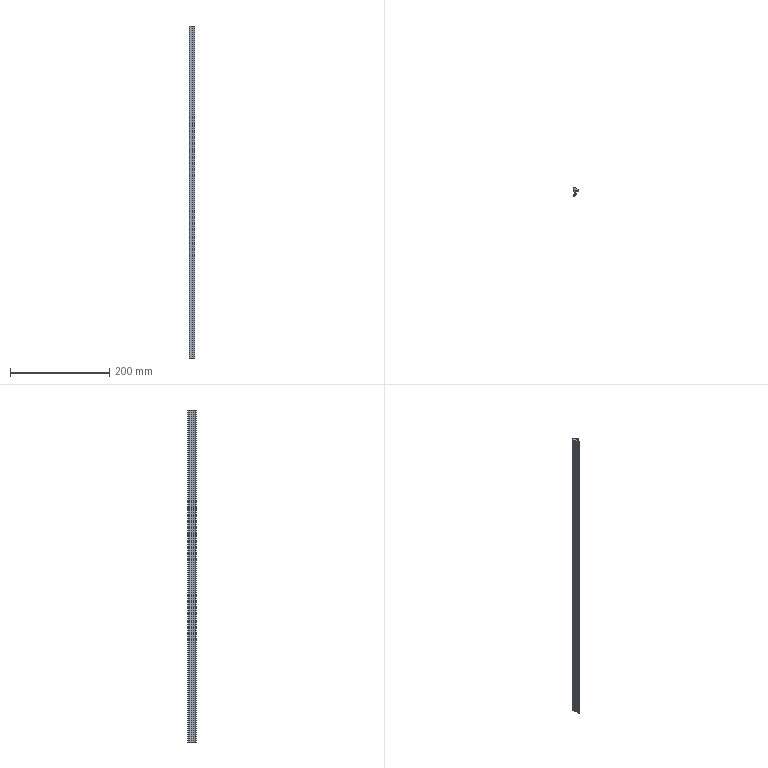Part | SolidWorks | features BaseBody 1, MoveFace 1 | 1 solid | 20 faces | box 10.8 x 17.5 x 670 mm | volume 52796 mm3 | cylinder 11 | plane 9 | commonest cylinder face diameters 1.6 x2 14 x2 0.4 x1 0.6 x1 0.8 x1 2.6 x1
STEP:
#1=CARTESIAN_POINT('',(-3.236,-11.055,570.));
#2=VERTEX_POINT('',#1);
#3=CARTESIAN_POINT('',(-4.3,-10.3,570.));
#4=VERTEX_POINT('',#3);
#5=CARTESIAN_POINT('',(-3.5,-10.3,570.));
#6=DIRECTION('',(0.,0.,-1.));
#7=DIRECTION('',(1.,0.,0.));
#8=AXIS2_PLACEMENT_3D('',#5,#6,#7);
#9=CIRCLE('',#8,0.8);
#10=EDGE_CURVE('',#2,#4,#9,.T.);
#11=ORIENTED_EDGE('',*,*,#10,.T.);
#12=CARTESIAN_POINT('',(-4.3,-10.3,-100.));
#13=VERTEX_POINT('',#12);
#14=CARTESIAN_POINT('',(-4.3,-10.3,-100.));
#15=DIRECTION('',(0.,0.,-1.));
#16=VECTOR('',#15,1000.);
#17=LINE('',#14,#16);
#18=EDGE_CURVE('',#4,#13,#17,.T.);
#19=ORIENTED_EDGE('',*,*,#18,.T.);
#20=CARTESIAN_POINT('',(-3.236,-11.055,-100.));
#21=VERTEX_POINT('',#20);
#22=CARTESIAN_POINT('',(-3.5,-10.3,-100.));
#23=DIRECTION('',(0.,0.,1.));
#24=DIRECTION('',(-1.,0.,0.));
#25=AXIS2_PLACEMENT_3D('',#22,#23,#24);
#26=CIRCLE('',#25,0.8);
#27=EDGE_CURVE('',#13,#21,#26,.T.);
#28=ORIENTED_EDGE('',*,*,#27,.T.);
#29=CARTESIAN_POINT('',(-3.236,-11.055,-100.));
#30=DIRECTION('',(0.,0.,-1.));
#31=VECTOR('',#30,1000.);
#32=LINE('',#29,#31);
#33=EDGE_CURVE('',#2,#21,#32,.T.);
#34=ORIENTED_EDGE('',*,*,#33,.F.);
#35=EDGE_LOOP('',(#11,#19,#28,#34));
#36=FACE_OUTER_BOUND('',#35,.T.);
#37=CARTESIAN_POINT('',(-3.5,-10.3,-100.));
#38=DIRECTION('',(0.,0.,-1.));
#39=DIRECTION('',(-1.,0.,0.));
#40=AXIS2_PLACEMENT_3D('',#37,#38,#39);
#41=CYLINDRICAL_SURFACE('',#40,0.8);
#42=ADVANCED_FACE('',(#36),#41,.T.);
#43=CARTESIAN_POINT('',(1.184,-6.397,-100.));
#44=VERTEX_POINT('',#43);
#45=CARTESIAN_POINT('',(-5.702,-4.29,-100.));
#46=DIRECTION('',(0.,0.,1.));
#47=DIRECTION('',(-1.,0.,0.));
#48=AXIS2_PLACEMENT_3D('',#45,#46,#47);
#49=CIRCLE('',#48,7.201);
#50=EDGE_CURVE('',#21,#44,#49,.T.);
#51=ORIENTED_EDGE('',*,*,#50,.T.);
#52=CARTESIAN_POINT('',(1.184,-6.397,570.));
#53=VERTEX_POINT('',#52);
#54=CARTESIAN_POINT('',(1.184,-6.397,-100.));
#55=DIRECTION('',(0.,0.,1.));
#56=VECTOR('',#55,1000.);
#57=LINE('',#54,#56);
#58=EDGE_CURVE('',#44,#53,#57,.T.);
#59=ORIENTED_EDGE('',*,*,#58,.T.);
#60=CARTESIAN_POINT('',(-5.702,-4.29,570.));
#61=DIRECTION('',(0.,0.,-1.));
#62=DIRECTION('',(1.,0.,0.));
#63=AXIS2_PLACEMENT_3D('',#60,#61,#62);
#64=CIRCLE('',#63,7.201);
#65=EDGE_CURVE('',#53,#2,#64,.T.);
#66=ORIENTED_EDGE('',*,*,#65,.T.);
#67=ORIENTED_EDGE('',*,*,#33,.T.);
#68=EDGE_LOOP('',(#51,#59,#66,#67));
#69=FACE_OUTER_BOUND('',#68,.T.);
#70=CARTESIAN_POINT('',(-5.702,-4.29,-100.));
#71=DIRECTION('',(0.,0.,-1.));
#72=DIRECTION('',(-1.,0.,0.));
#73=AXIS2_PLACEMENT_3D('',#70,#71,#72);
#74=CYLINDRICAL_SURFACE('',#73,7.201);
#75=ADVANCED_FACE('',(#69),#74,.T.);
#76=CARTESIAN_POINT('',(0.9,-6.,-100.));
#77=VERTEX_POINT('',#76);
#78=CARTESIAN_POINT('',(0.9,-6.3,-100.));
#79=DIRECTION('',(0.,0.,1.));
#80=DIRECTION('',(-1.,0.,0.));
#81=AXIS2_PLACEMENT_3D('',#78,#79,#80);
#82=CIRCLE('',#81,0.3);
#83=EDGE_CURVE('',#44,#77,#82,.T.);
#84=ORIENTED_EDGE('',*,*,#83,.T.);
#85=CARTESIAN_POINT('',(0.9,-6.,570.));
#86=VERTEX_POINT('',#85);
#87=CARTESIAN_POINT('',(0.9,-6.,-100.));
#88=DIRECTION('',(0.,0.,1.));
#89=VECTOR('',#88,1000.);
#90=LINE('',#87,#89);
#91=EDGE_CURVE('',#77,#86,#90,.T.);
#92=ORIENTED_EDGE('',*,*,#91,.T.);
#93=CARTESIAN_POINT('',(0.9,-6.3,570.));
#94=DIRECTION('',(0.,0.,-1.));
#95=DIRECTION('',(1.,0.,0.));
#96=AXIS2_PLACEMENT_3D('',#93,#94,#95);
#97=CIRCLE('',#96,0.3);
#98=EDGE_CURVE('',#86,#53,#97,.T.);
#99=ORIENTED_EDGE('',*,*,#98,.T.);
#100=ORIENTED_EDGE('',*,*,#58,.F.);
#101=EDGE_LOOP('',(#84,#92,#99,#100));
#102=FACE_OUTER_BOUND('',#101,.T.);
#103=CARTESIAN_POINT('',(0.9,-6.3,-100.));
#104=DIRECTION('',(0.,0.,-1.));
#105=DIRECTION('',(-1.,0.,0.));
#106=AXIS2_PLACEMENT_3D('',#103,#104,#105);
#107=CYLINDRICAL_SURFACE('',#106,0.3);
#108=ADVANCED_FACE('',(#102),#107,.T.);
#109=CARTESIAN_POINT('',(-2.5,-0.5,-100.));
#110=VERTEX_POINT('',#109);
#111=CARTESIAN_POINT('',(-2.5,-6.153,-100.));
#112=VERTEX_POINT('',#111);
#113=CARTESIAN_POINT('',(-2.5,-6.397,-100.));
#114=DIRECTION('',(0.,-1.,0.));
#115=VECTOR('',#114,1000.);
#116=LINE('',#113,#115);
#117=EDGE_CURVE('',#110,#112,#116,.T.);
#118=ORIENTED_EDGE('',*,*,#117,.F.);
#119=CARTESIAN_POINT('',(-4.2,1.695,-100.));
#120=VERTEX_POINT('',#119);
#121=CARTESIAN_POINT('',(-1.701,1.875,-100.));
#122=DIRECTION('',(0.,0.,1.));
#123=DIRECTION('',(-1.,0.,0.));
#124=AXIS2_PLACEMENT_3D('',#121,#122,#123);
#125=CIRCLE('',#124,2.506);
#126=EDGE_CURVE('',#120,#110,#125,.T.);
#127=ORIENTED_EDGE('',*,*,#126,.F.);
#128=CARTESIAN_POINT('',(-4.2,5.1,-100.));
#129=VERTEX_POINT('',#128);
#130=CARTESIAN_POINT('',(-4.2,-6.397,-100.));
#131=DIRECTION('',(0.,-1.,0.));
#132=VECTOR('',#131,1000.);
#133=LINE('',#130,#132);
#134=EDGE_CURVE('',#129,#120,#133,.T.);
#135=ORIENTED_EDGE('',*,*,#134,.F.);
#136=CARTESIAN_POINT('',(-2.892,6.4,-100.));
#137=VERTEX_POINT('',#136);
#138=CARTESIAN_POINT('',(-2.9,5.1,-100.));
#139=DIRECTION('',(0.,0.,1.));
#140=DIRECTION('',(-1.,0.,0.));
#141=AXIS2_PLACEMENT_3D('',#138,#139,#140);
#142=CIRCLE('',#141,1.3);
#143=EDGE_CURVE('',#137,#129,#142,.T.);
#144=ORIENTED_EDGE('',*,*,#143,.F.);
#145=CARTESIAN_POINT('',(0.5,5.5,-100.));
#146=VERTEX_POINT('',#145);
#147=CARTESIAN_POINT('',(-2.934,-0.5999,-100.));
#148=DIRECTION('',(0.,0.,1.));
#149=DIRECTION('',(-1.,0.,0.));
#150=AXIS2_PLACEMENT_3D('',#147,#148,#149);
#151=CIRCLE('',#150,7.);
#152=EDGE_CURVE('',#146,#137,#151,.T.);
#153=ORIENTED_EDGE('',*,*,#152,.F.);
#154=CARTESIAN_POINT('',(5.5,1.7,-100.));
#155=VERTEX_POINT('',#154);
#156=CARTESIAN_POINT('',(5.5,1.7,-100.));
#157=DIRECTION('',(-0.7962,0.6051,0.));
#158=VECTOR('',#157,1000.);
#159=LINE('',#156,#158);
#160=EDGE_CURVE('',#155,#146,#159,.T.);
#161=ORIENTED_EDGE('',*,*,#160,.F.);
#162=CARTESIAN_POINT('',(6.458,-0.2215,-100.));
#163=VERTEX_POINT('',#162);
#164=CARTESIAN_POINT('',(6.458,-0.2215,-100.));
#165=DIRECTION('',(-0.4462,0.8949,0.));
#166=VECTOR('',#165,1000.);
#167=LINE('',#164,#166);
#168=EDGE_CURVE('',#163,#155,#167,.T.);
#169=ORIENTED_EDGE('',*,*,#168,.F.);
#170=CARTESIAN_POINT('',(5.895,-0.7433,-100.));
#171=VERTEX_POINT('',#170);
#172=CARTESIAN_POINT('',(6.1,-0.4,-100.));
#173=DIRECTION('',(0.,0.,1.));
#174=DIRECTION('',(-1.,0.,0.));
#175=AXIS2_PLACEMENT_3D('',#172,#173,#174);
#176=CIRCLE('',#175,0.4);
#177=EDGE_CURVE('',#171,#163,#176,.T.);
#178=ORIENTED_EDGE('',*,*,#177,.F.);
#179=CARTESIAN_POINT('',(3.,0.,-100.));
#180=VERTEX_POINT('',#179);
#181=CARTESIAN_POINT('',(2.746,-6.995,-100.));
#182=DIRECTION('',(0.,0.,-1.));
#183=DIRECTION('',(-1.,0.,0.));
#184=AXIS2_PLACEMENT_3D('',#181,#182,#183);
#185=CIRCLE('',#184,7.);
#186=EDGE_CURVE('',#180,#171,#185,.T.);
#187=ORIENTED_EDGE('',*,*,#186,.F.);
#188=CARTESIAN_POINT('',(0.,0.,-100.));
#189=VERTEX_POINT('',#188);
#190=CARTESIAN_POINT('',(-6.814,0.,-100.));
#191=DIRECTION('',(1.,0.,0.));
#192=VECTOR('',#191,1000.);
#193=LINE('',#190,#192);
#194=EDGE_CURVE('',#189,#180,#193,.T.);
#195=ORIENTED_EDGE('',*,*,#194,.F.);
#196=CARTESIAN_POINT('',(0.,-5.8,-100.));
#197=VERTEX_POINT('',#196);
#198=CARTESIAN_POINT('',(0.,-6.397,-100.));
#199=DIRECTION('',(0.,1.,0.));
#200=VECTOR('',#199,1000.);
#201=LINE('',#198,#200);
#202=EDGE_CURVE('',#197,#189,#201,.T.);
#203=ORIENTED_EDGE('',*,*,#202,.F.);
#204=CARTESIAN_POINT('',(0.2,-6.,-100.));
#205=VERTEX_POINT('',#204);
#206=CARTESIAN_POINT('',(0.2,-5.8,-100.));
#207=DIRECTION('',(0.,0.,1.));
#208=DIRECTION('',(-1.,0.,0.));
#209=AXIS2_PLACEMENT_3D('',#206,#207,#208);
#210=CIRCLE('',#209,0.2);
#211=EDGE_CURVE('',#197,#205,#210,.T.);
#212=ORIENTED_EDGE('',*,*,#211,.T.);
#213=CARTESIAN_POINT('',(-6.814,-6.,-100.));
#214=DIRECTION('',(-1.,0.,0.));
#215=VECTOR('',#214,1000.);
#216=LINE('',#213,#215);
#217=EDGE_CURVE('',#77,#205,#216,.T.);
#218=ORIENTED_EDGE('',*,*,#217,.F.);
#219=ORIENTED_EDGE('',*,*,#83,.F.);
#220=ORIENTED_EDGE('',*,*,#50,.F.);
#221=ORIENTED_EDGE('',*,*,#27,.F.);
#222=CARTESIAN_POINT('',(-3.998,-9.674,-100.));
#223=VERTEX_POINT('',#222);
#224=CARTESIAN_POINT('',(-3.5,-10.3,-100.));
#225=DIRECTION('',(0.,0.,1.));
#226=DIRECTION('',(-1.,0.,0.));
#227=AXIS2_PLACEMENT_3D('',#224,#225,#226);
#228=CIRCLE('',#227,0.8);
#229=EDGE_CURVE('',#223,#13,#228,.T.);
#230=ORIENTED_EDGE('',*,*,#229,.F.);
#231=CARTESIAN_POINT('',(-6.814,-6.397,-100.));
#232=DIRECTION('',(0.,0.,-1.));
#233=DIRECTION('',(-1.,0.,0.));
#234=AXIS2_PLACEMENT_3D('',#231,#232,#233);
#235=CIRCLE('',#234,4.321);
#236=EDGE_CURVE('',#112,#223,#235,.T.);
#237=ORIENTED_EDGE('',*,*,#236,.F.);
#238=EDGE_LOOP('',(#118,#127,#135,#144,#153,#161,#169,#178,#187,#195,#203,#212,#218,#219,#220,#221,#230,#237));
#239=FACE_OUTER_BOUND('',#238,.T.);
#240=CARTESIAN_POINT('',(-6.814,-6.397,-100.));
#241=DIRECTION('',(0.,0.,1.));
#242=DIRECTION('',(1.,0.,0.));
#243=AXIS2_PLACEMENT_3D('',#240,#241,#242);
#244=PLANE('',#243);
#245=ADVANCED_FACE('',(#239),#244,.F.);
#246=ORIENTED_EDGE('',*,*,#18,.F.);
#247=CARTESIAN_POINT('',(-3.998,-9.674,570.));
#248=VERTEX_POINT('',#247);
#249=CARTESIAN_POINT('',(-3.5,-10.3,570.));
#250=DIRECTION('',(0.,0.,-1.));
#251=DIRECTION('',(1.,0.,0.));
#252=AXIS2_PLACEMENT_3D('',#249,#250,#251);
#253=CIRCLE('',#252,0.8);
#254=EDGE_CURVE('',#4,#248,#253,.T.);
#255=ORIENTED_EDGE('',*,*,#254,.T.);
#256=CARTESIAN_POINT('',(-3.998,-9.674,-100.));
#257=DIRECTION('',(0.,0.,-1.));
#258=VECTOR('',#257,1000.);
#259=LINE('',#256,#258);
#260=EDGE_CURVE('',#248,#223,#259,.T.);
#261=ORIENTED_EDGE('',*,*,#260,.T.);
#262=ORIENTED_EDGE('',*,*,#229,.T.);
#263=EDGE_LOOP('',(#246,#255,#261,#262));
#264=FACE_OUTER_BOUND('',#263,.T.);
#265=CARTESIAN_POINT('',(-3.5,-10.3,-100.));
#266=DIRECTION('',(0.,0.,-1.));
#267=DIRECTION('',(-1.,0.,0.));
#268=AXIS2_PLACEMENT_3D('',#265,#266,#267);
#269=CYLINDRICAL_SURFACE('',#268,0.8);
#270=ADVANCED_FACE('',(#264),#269,.T.);
#271=CARTESIAN_POINT('',(-4.2,1.695,570.));
#272=VERTEX_POINT('',#271);
#273=CARTESIAN_POINT('',(-2.5,-0.5,570.));
#274=VERTEX_POINT('',#273);
#275=CARTESIAN_POINT('',(-1.701,1.875,570.));
#276=DIRECTION('',(0.,0.,1.));
#277=DIRECTION('',(1.,0.,0.));
#278=AXIS2_PLACEMENT_3D('',#275,#276,#277);
#279=CIRCLE('',#278,2.506);
#280=EDGE_CURVE('',#272,#274,#279,.T.);
#281=ORIENTED_EDGE('',*,*,#280,.T.);
#282=CARTESIAN_POINT('',(-2.5,-6.153,570.));
#283=VERTEX_POINT('',#282);
#284=CARTESIAN_POINT('',(-2.5,-6.397,570.));
#285=DIRECTION('',(0.,-1.,0.));
#286=VECTOR('',#285,1000.);
#287=LINE('',#284,#286);
#288=EDGE_CURVE('',#274,#283,#287,.T.);
#289=ORIENTED_EDGE('',*,*,#288,.T.);
#290=CARTESIAN_POINT('',(-6.814,-6.397,570.));
#291=DIRECTION('',(0.,0.,-1.));
#292=DIRECTION('',(1.,0.,0.));
#293=AXIS2_PLACEMENT_3D('',#290,#291,#292);
#294=CIRCLE('',#293,4.321);
#295=EDGE_CURVE('',#283,#248,#294,.T.);
#296=ORIENTED_EDGE('',*,*,#295,.T.);
#297=ORIENTED_EDGE('',*,*,#254,.F.);
#298=ORIENTED_EDGE('',*,*,#10,.F.);
#299=ORIENTED_EDGE('',*,*,#65,.F.);
#300=ORIENTED_EDGE('',*,*,#98,.F.);
#301=CARTESIAN_POINT('',(0.2,-6.,570.));
#302=VERTEX_POINT('',#301);
#303=CARTESIAN_POINT('',(-6.814,-6.,570.));
#304=DIRECTION('',(-1.,0.,0.));
#305=VECTOR('',#304,1000.);
#306=LINE('',#303,#305);
#307=EDGE_CURVE('',#86,#302,#306,.T.);
#308=ORIENTED_EDGE('',*,*,#307,.T.);
#309=CARTESIAN_POINT('',(0.,-5.8,570.));
#310=VERTEX_POINT('',#309);
#311=CARTESIAN_POINT('',(0.2,-5.8,570.));
#312=DIRECTION('',(0.,0.,-1.));
#313=DIRECTION('',(1.,0.,0.));
#314=AXIS2_PLACEMENT_3D('',#311,#312,#313);
#315=CIRCLE('',#314,0.2);
#316=EDGE_CURVE('',#302,#310,#315,.T.);
#317=ORIENTED_EDGE('',*,*,#316,.T.);
#318=CARTESIAN_POINT('',(0.,0.,570.));
#319=VERTEX_POINT('',#318);
#320=CARTESIAN_POINT('',(0.,-6.397,570.));
#321=DIRECTION('',(0.,1.,0.));
#322=VECTOR('',#321,1000.);
#323=LINE('',#320,#322);
#324=EDGE_CURVE('',#310,#319,#323,.T.);
#325=ORIENTED_EDGE('',*,*,#324,.T.);
#326=CARTESIAN_POINT('',(3.,0.,570.));
#327=VERTEX_POINT('',#326);
#328=CARTESIAN_POINT('',(-6.814,0.,570.));
#329=DIRECTION('',(1.,0.,0.));
#330=VECTOR('',#329,1000.);
#331=LINE('',#328,#330);
#332=EDGE_CURVE('',#319,#327,#331,.T.);
#333=ORIENTED_EDGE('',*,*,#332,.T.);
#334=CARTESIAN_POINT('',(5.895,-0.7433,570.));
#335=VERTEX_POINT('',#334);
#336=CARTESIAN_POINT('',(2.746,-6.995,570.));
#337=DIRECTION('',(0.,0.,-1.));
#338=DIRECTION('',(1.,0.,0.));
#339=AXIS2_PLACEMENT_3D('',#336,#337,#338);
#340=CIRCLE('',#339,7.);
#341=EDGE_CURVE('',#327,#335,#340,.T.);
#342=ORIENTED_EDGE('',*,*,#341,.T.);
#343=CARTESIAN_POINT('',(6.458,-0.2215,570.));
#344=VERTEX_POINT('',#343);
#345=CARTESIAN_POINT('',(6.1,-0.4,570.));
#346=DIRECTION('',(0.,0.,-1.));
#347=DIRECTION('',(1.,0.,0.));
#348=AXIS2_PLACEMENT_3D('',#345,#346,#347);
#349=CIRCLE('',#348,0.4);
#350=EDGE_CURVE('',#344,#335,#349,.T.);
#351=ORIENTED_EDGE('',*,*,#350,.F.);
#352=CARTESIAN_POINT('',(5.5,1.7,570.));
#353=VERTEX_POINT('',#352);
#354=CARTESIAN_POINT('',(6.282,0.1323,570.));
#355=DIRECTION('',(-0.4462,0.8949,0.));
#356=VECTOR('',#355,1000.);
#357=LINE('',#354,#356);
#358=EDGE_CURVE('',#344,#353,#357,.T.);
#359=ORIENTED_EDGE('',*,*,#358,.T.);
#360=CARTESIAN_POINT('',(0.5,5.5,570.));
#361=VERTEX_POINT('',#360);
#362=CARTESIAN_POINT('',(1.595,4.668,570.));
#363=DIRECTION('',(-0.7962,0.6051,0.));
#364=VECTOR('',#363,1000.);
#365=LINE('',#362,#364);
#366=EDGE_CURVE('',#353,#361,#365,.T.);
#367=ORIENTED_EDGE('',*,*,#366,.T.);
#368=CARTESIAN_POINT('',(-2.892,6.4,570.));
#369=VERTEX_POINT('',#368);
#370=CARTESIAN_POINT('',(-2.934,-0.5999,570.));
#371=DIRECTION('',(0.,0.,1.));
#372=DIRECTION('',(1.,0.,0.));
#373=AXIS2_PLACEMENT_3D('',#370,#371,#372);
#374=CIRCLE('',#373,7.);
#375=EDGE_CURVE('',#361,#369,#374,.T.);
#376=ORIENTED_EDGE('',*,*,#375,.T.);
#377=CARTESIAN_POINT('',(-4.2,5.1,570.));
#378=VERTEX_POINT('',#377);
#379=CARTESIAN_POINT('',(-2.9,5.1,570.));
#380=DIRECTION('',(0.,0.,1.));
#381=DIRECTION('',(1.,0.,0.));
#382=AXIS2_PLACEMENT_3D('',#379,#380,#381);
#383=CIRCLE('',#382,1.3);
#384=EDGE_CURVE('',#369,#378,#383,.T.);
#385=ORIENTED_EDGE('',*,*,#384,.T.);
#386=CARTESIAN_POINT('',(-4.2,-6.397,570.));
#387=DIRECTION('',(0.,-1.,0.));
#388=VECTOR('',#387,1000.);
#389=LINE('',#386,#388);
#390=EDGE_CURVE('',#378,#272,#389,.T.);
#391=ORIENTED_EDGE('',*,*,#390,.T.);
#392=EDGE_LOOP('',(#281,#289,#296,#297,#298,#299,#300,#308,#317,#325,#333,#342,#351,#359,#367,#376,#385,#391));
#393=FACE_OUTER_BOUND('',#392,.T.);
#394=CARTESIAN_POINT('',(-6.814,-6.397,570.));
#395=DIRECTION('',(0.,0.,1.));
#396=DIRECTION('',(1.,0.,0.));
#397=AXIS2_PLACEMENT_3D('',#394,#395,#396);
#398=PLANE('',#397);
#399=ADVANCED_FACE('',(#393),#398,.T.);
#400=ORIENTED_EDGE('',*,*,#217,.T.);
#401=CARTESIAN_POINT('',(0.2,-6.,-100.));
#402=DIRECTION('',(0.,0.,1.));
#403=VECTOR('',#402,1000.);
#404=LINE('',#401,#403);
#405=EDGE_CURVE('',#205,#302,#404,.T.);
#406=ORIENTED_EDGE('',*,*,#405,.T.);
#407=ORIENTED_EDGE('',*,*,#307,.F.);
#408=ORIENTED_EDGE('',*,*,#91,.F.);
#409=EDGE_LOOP('',(#400,#406,#407,#408));
#410=FACE_OUTER_BOUND('',#409,.T.);
#411=CARTESIAN_POINT('',(0.9,-6.,-100.));
#412=DIRECTION('',(0.,1.,0.));
#413=DIRECTION('',(0.,0.,1.));
#414=AXIS2_PLACEMENT_3D('',#411,#412,#413);
#415=PLANE('',#414);
#416=ADVANCED_FACE('',(#410),#415,.T.);
#417=CARTESIAN_POINT('',(-2.5,-6.153,-100.));
#418=DIRECTION('',(0.,0.,1.));
#419=VECTOR('',#418,1000.);
#420=LINE('',#417,#419);
#421=EDGE_CURVE('',#112,#283,#420,.T.);
#422=ORIENTED_EDGE('',*,*,#421,.F.);
#423=ORIENTED_EDGE('',*,*,#236,.T.);
#424=ORIENTED_EDGE('',*,*,#260,.F.);
#425=ORIENTED_EDGE('',*,*,#295,.F.);
#426=EDGE_LOOP('',(#422,#423,#424,#425));
#427=FACE_OUTER_BOUND('',#426,.T.);
#428=CARTESIAN_POINT('',(-6.814,-6.397,-100.));
#429=DIRECTION('',(0.,0.,-1.));
#430=DIRECTION('',(-1.,0.,0.));
#431=AXIS2_PLACEMENT_3D('',#428,#429,#430);
#432=CYLINDRICAL_SURFACE('',#431,4.321);
#433=ADVANCED_FACE('',(#427),#432,.F.);
#434=ORIENTED_EDGE('',*,*,#117,.T.);
#435=ORIENTED_EDGE('',*,*,#421,.T.);
#436=ORIENTED_EDGE('',*,*,#288,.F.);
#437=CARTESIAN_POINT('',(-2.5,-0.5,-100.));
#438=DIRECTION('',(0.,0.,-1.));
#439=VECTOR('',#438,1000.);
#440=LINE('',#437,#439);
#441=EDGE_CURVE('',#274,#110,#440,.T.);
#442=ORIENTED_EDGE('',*,*,#441,.T.);
#443=EDGE_LOOP('',(#434,#435,#436,#442));
#444=FACE_OUTER_BOUND('',#443,.T.);
#445=CARTESIAN_POINT('',(-2.5,-0.5,-100.));
#446=DIRECTION('',(-1.,0.,0.));
#447=DIRECTION('',(0.,0.,1.));
#448=AXIS2_PLACEMENT_3D('',#445,#446,#447);
#449=PLANE('',#448);
#450=ADVANCED_FACE('',(#444),#449,.T.);
#451=ORIENTED_EDGE('',*,*,#126,.T.);
#452=ORIENTED_EDGE('',*,*,#441,.F.);
#453=ORIENTED_EDGE('',*,*,#280,.F.);
#454=CARTESIAN_POINT('',(-4.2,1.695,-100.));
#455=DIRECTION('',(0.,0.,-1.));
#456=VECTOR('',#455,1000.);
#457=LINE('',#454,#456);
#458=EDGE_CURVE('',#272,#120,#457,.T.);
#459=ORIENTED_EDGE('',*,*,#458,.T.);
#460=EDGE_LOOP('',(#451,#452,#453,#459));
#461=FACE_OUTER_BOUND('',#460,.T.);
#462=CARTESIAN_POINT('',(-1.701,1.875,-100.));
#463=DIRECTION('',(0.,0.,-1.));
#464=DIRECTION('',(-1.,0.,0.));
#465=AXIS2_PLACEMENT_3D('',#462,#463,#464);
#466=CYLINDRICAL_SURFACE('',#465,2.506);
#467=ADVANCED_FACE('',(#461),#466,.T.);
#468=ORIENTED_EDGE('',*,*,#134,.T.);
#469=ORIENTED_EDGE('',*,*,#458,.F.);
#470=ORIENTED_EDGE('',*,*,#390,.F.);
#471=CARTESIAN_POINT('',(-4.2,5.1,-100.));
#472=DIRECTION('',(0.,0.,-1.));
#473=VECTOR('',#472,1000.);
#474=LINE('',#471,#473);
#475=EDGE_CURVE('',#378,#129,#474,.T.);
#476=ORIENTED_EDGE('',*,*,#475,.T.);
#477=EDGE_LOOP('',(#468,#469,#470,#476));
#478=FACE_OUTER_BOUND('',#477,.T.);
#479=CARTESIAN_POINT('',(-4.2,5.1,-100.));
#480=DIRECTION('',(-1.,0.,0.));
#481=DIRECTION('',(0.,0.,1.));
#482=AXIS2_PLACEMENT_3D('',#479,#480,#481);
#483=PLANE('',#482);
#484=ADVANCED_FACE('',(#478),#483,.T.);
#485=ORIENTED_EDGE('',*,*,#143,.T.);
#486=ORIENTED_EDGE('',*,*,#475,.F.);
#487=ORIENTED_EDGE('',*,*,#384,.F.);
#488=CARTESIAN_POINT('',(-2.892,6.4,-100.));
#489=DIRECTION('',(0.,0.,-1.));
#490=VECTOR('',#489,1000.);
#491=LINE('',#488,#490);
#492=EDGE_CURVE('',#369,#137,#491,.T.);
#493=ORIENTED_EDGE('',*,*,#492,.T.);
#494=EDGE_LOOP('',(#485,#486,#487,#493));
#495=FACE_OUTER_BOUND('',#494,.T.);
#496=CARTESIAN_POINT('',(-2.9,5.1,-100.));
#497=DIRECTION('',(0.,0.,-1.));
#498=DIRECTION('',(-1.,0.,0.));
#499=AXIS2_PLACEMENT_3D('',#496,#497,#498);
#500=CYLINDRICAL_SURFACE('',#499,1.3);
#501=ADVANCED_FACE('',(#495),#500,.T.);
#502=ORIENTED_EDGE('',*,*,#152,.T.);
#503=ORIENTED_EDGE('',*,*,#492,.F.);
#504=ORIENTED_EDGE('',*,*,#375,.F.);
#505=CARTESIAN_POINT('',(0.5,5.5,-100.));
#506=DIRECTION('',(0.,0.,-1.));
#507=VECTOR('',#506,1000.);
#508=LINE('',#505,#507);
#509=EDGE_CURVE('',#361,#146,#508,.T.);
#510=ORIENTED_EDGE('',*,*,#509,.T.);
#511=EDGE_LOOP('',(#502,#503,#504,#510));
#512=FACE_OUTER_BOUND('',#511,.T.);
#513=CARTESIAN_POINT('',(-2.934,-0.5999,-100.));
#514=DIRECTION('',(0.,0.,-1.));
#515=DIRECTION('',(-1.,0.,0.));
#516=AXIS2_PLACEMENT_3D('',#513,#514,#515);
#517=CYLINDRICAL_SURFACE('',#516,7.);
#518=ADVANCED_FACE('',(#512),#517,.T.);
#519=ORIENTED_EDGE('',*,*,#160,.T.);
#520=ORIENTED_EDGE('',*,*,#509,.F.);
#521=ORIENTED_EDGE('',*,*,#366,.F.);
#522=CARTESIAN_POINT('',(5.5,1.7,-100.));
#523=DIRECTION('',(0.,0.,-1.));
#524=VECTOR('',#523,1000.);
#525=LINE('',#522,#524);
#526=EDGE_CURVE('',#353,#155,#525,.T.);
#527=ORIENTED_EDGE('',*,*,#526,.T.);
#528=EDGE_LOOP('',(#519,#520,#521,#527));
#529=FACE_OUTER_BOUND('',#528,.T.);
#530=CARTESIAN_POINT('',(5.5,1.7,-100.));
#531=DIRECTION('',(0.6051,0.7962,0.));
#532=DIRECTION('',(-0.7962,0.6051,0.));
#533=AXIS2_PLACEMENT_3D('',#530,#531,#532);
#534=PLANE('',#533);
#535=ADVANCED_FACE('',(#529),#534,.T.);
#536=ORIENTED_EDGE('',*,*,#168,.T.);
#537=ORIENTED_EDGE('',*,*,#526,.F.);
#538=ORIENTED_EDGE('',*,*,#358,.F.);
#539=CARTESIAN_POINT('',(6.458,-0.2215,-100.));
#540=DIRECTION('',(0.,0.,-1.));
#541=VECTOR('',#540,1000.);
#542=LINE('',#539,#541);
#543=EDGE_CURVE('',#344,#163,#542,.T.);
#544=ORIENTED_EDGE('',*,*,#543,.T.);
#545=EDGE_LOOP('',(#536,#537,#538,#544));
#546=FACE_OUTER_BOUND('',#545,.T.);
#547=CARTESIAN_POINT('',(6.458,-0.2215,-100.));
#548=DIRECTION('',(0.8949,0.4462,0.));
#549=DIRECTION('',(-0.4462,0.8949,0.));
#550=AXIS2_PLACEMENT_3D('',#547,#548,#549);
#551=PLANE('',#550);
#552=ADVANCED_FACE('',(#546),#551,.T.);
#553=CARTESIAN_POINT('',(3.,0.,-100.));
#554=DIRECTION('',(0.,0.,1.));
#555=VECTOR('',#554,1000.);
#556=LINE('',#553,#555);
#557=EDGE_CURVE('',#180,#327,#556,.T.);
#558=ORIENTED_EDGE('',*,*,#557,.F.);
#559=ORIENTED_EDGE('',*,*,#186,.T.);
#560=CARTESIAN_POINT('',(5.895,-0.7433,-100.));
#561=DIRECTION('',(0.,0.,-1.));
#562=VECTOR('',#561,1000.);
#563=LINE('',#560,#562);
#564=EDGE_CURVE('',#335,#171,#563,.T.);
#565=ORIENTED_EDGE('',*,*,#564,.F.);
#566=ORIENTED_EDGE('',*,*,#341,.F.);
#567=EDGE_LOOP('',(#558,#559,#565,#566));
#568=FACE_OUTER_BOUND('',#567,.T.);
#569=CARTESIAN_POINT('',(2.746,-6.995,-100.));
#570=DIRECTION('',(0.,0.,-1.));
#571=DIRECTION('',(-1.,0.,0.));
#572=AXIS2_PLACEMENT_3D('',#569,#570,#571);
#573=CYLINDRICAL_SURFACE('',#572,7.);
#574=ADVANCED_FACE('',(#568),#573,.F.);
#575=ORIENTED_EDGE('',*,*,#194,.T.);
#576=ORIENTED_EDGE('',*,*,#557,.T.);
#577=ORIENTED_EDGE('',*,*,#332,.F.);
#578=CARTESIAN_POINT('',(0.,0.,-100.));
#579=DIRECTION('',(0.,0.,-1.));
#580=VECTOR('',#579,1000.);
#581=LINE('',#578,#580);
#582=EDGE_CURVE('',#319,#189,#581,.T.);
#583=ORIENTED_EDGE('',*,*,#582,.T.);
#584=EDGE_LOOP('',(#575,#576,#577,#583));
#585=FACE_OUTER_BOUND('',#584,.T.);
#586=CARTESIAN_POINT('',(0.,0.,-100.));
#587=DIRECTION('',(0.,-1.,0.));
#588=DIRECTION('',(0.,0.,-1.));
#589=AXIS2_PLACEMENT_3D('',#586,#587,#588);
#590=PLANE('',#589);
#591=ADVANCED_FACE('',(#585),#590,.T.);
#592=ORIENTED_EDGE('',*,*,#202,.T.);
#593=ORIENTED_EDGE('',*,*,#582,.F.);
#594=ORIENTED_EDGE('',*,*,#324,.F.);
#595=CARTESIAN_POINT('',(0.,-5.8,-100.));
#596=DIRECTION('',(0.,0.,-1.));
#597=VECTOR('',#596,1000.);
#598=LINE('',#595,#597);
#599=EDGE_CURVE('',#310,#197,#598,.T.);
#600=ORIENTED_EDGE('',*,*,#599,.T.);
#601=EDGE_LOOP('',(#592,#593,#594,#600));
#602=FACE_OUTER_BOUND('',#601,.T.);
#603=CARTESIAN_POINT('',(0.,-5.8,-100.));
#604=DIRECTION('',(1.,0.,0.));
#605=DIRECTION('',(0.,0.,-1.));
#606=AXIS2_PLACEMENT_3D('',#603,#604,#605);
#607=PLANE('',#606);
#608=ADVANCED_FACE('',(#602),#607,.T.);
#609=ORIENTED_EDGE('',*,*,#405,.F.);
#610=ORIENTED_EDGE('',*,*,#211,.F.);
#611=ORIENTED_EDGE('',*,*,#599,.F.);
#612=ORIENTED_EDGE('',*,*,#316,.F.);
#613=EDGE_LOOP('',(#609,#610,#611,#612));
#614=FACE_OUTER_BOUND('',#613,.T.);
#615=CARTESIAN_POINT('',(0.2,-5.8,-100.));
#616=DIRECTION('',(0.,0.,-1.));
#617=DIRECTION('',(-1.,0.,0.));
#618=AXIS2_PLACEMENT_3D('',#615,#616,#617);
#619=CYLINDRICAL_SURFACE('',#618,0.2);
#620=ADVANCED_FACE('',(#614),#619,.F.);
#621=ORIENTED_EDGE('',*,*,#177,.T.);
#622=ORIENTED_EDGE('',*,*,#543,.F.);
#623=ORIENTED_EDGE('',*,*,#350,.T.);
#624=ORIENTED_EDGE('',*,*,#564,.T.);
#625=EDGE_LOOP('',(#621,#622,#623,#624));
#626=FACE_OUTER_BOUND('',#625,.T.);
#627=CARTESIAN_POINT('',(6.1,-0.4,-100.));
#628=DIRECTION('',(0.,0.,-1.));
#629=DIRECTION('',(-1.,0.,0.));
#630=AXIS2_PLACEMENT_3D('',#627,#628,#629);
#631=CYLINDRICAL_SURFACE('',#630,0.4);
#632=ADVANCED_FACE('',(#626),#631,.T.);
#633=CLOSED_SHELL('',(#42,#75,#108,#245,#270,#399,#416,#433,#450,#467,#484,#501,#518,#535,#552,#574,#591,#608,#620,#632));
#634=MANIFOLD_SOLID_BREP('',#633);
#635=CARTESIAN_POINT('',(0.,0.,0.));
#636=DIRECTION('',(0.,0.,1.));
#637=DIRECTION('',(1.,0.,0.));
#638=AXIS2_PLACEMENT_3D('',#635,#636,#637);
#639=(LENGTH_UNIT()NAMED_UNIT(*)SI_UNIT(.MILLI.,.METRE.));
#640=UNCERTAINTY_MEASURE_WITH_UNIT(LENGTH_MEASURE(0.00001),#639,'','');
#641=(NAMED_UNIT(*)PLANE_ANGLE_UNIT()SI_UNIT($,.RADIAN.));
#642=(NAMED_UNIT(*)SI_UNIT($,.STERADIAN.)SOLID_ANGLE_UNIT());
#643=(GEOMETRIC_REPRESENTATION_CONTEXT(3)GLOBAL_UNCERTAINTY_ASSIGNED_CONTEXT((#640))GLOBAL_UNIT_ASSIGNED_CONTEXT((#639,#641,#642))REPRESENTATION_CONTEXT('',''));
#644=ADVANCED_BREP_SHAPE_REPRESENTATION('',(#634,#638),#643);